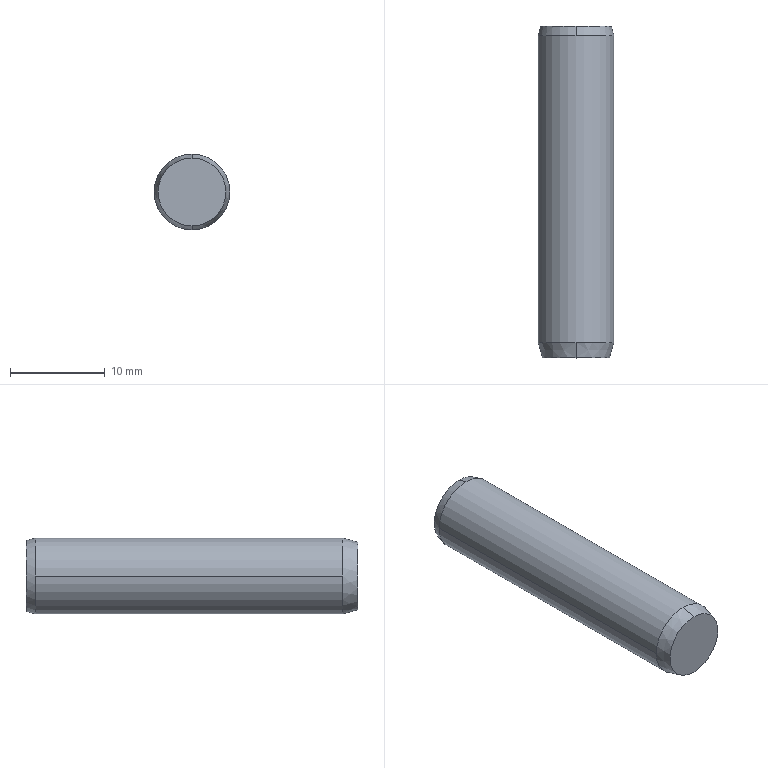Part | STEP file | 1 solid | 16 faces | box 8 x 35 x 8 mm | volume 1570 mm3 | cone 8 | cylinder 6 | plane 2 | commonest cylinder face diameters 4.134 x2 5.3 x2 8 x2
STEP:
#1=CARTESIAN_POINT('',(0.,-35.,3.571));
#2=VERTEX_POINT('',#1);
#3=CARTESIAN_POINT('',(0.,-35.,-3.571));
#4=VERTEX_POINT('',#3);
#5=CARTESIAN_POINT('',(0.,-35.,0.));
#6=DIRECTION('',(0.,1.,0.));
#7=DIRECTION('',(0.,0.,1.));
#8=AXIS2_PLACEMENT_3D('',#5,#6,#7);
#9=CIRCLE('',#8,3.571);
#10=EDGE_CURVE('',#2,#4,#9,.T.);
#11=ORIENTED_EDGE('',*,*,#10,.T.);
#12=CARTESIAN_POINT('',(0.,-33.4,-4.));
#13=VERTEX_POINT('',#12);
#14=CARTESIAN_POINT('',(0.,-35.,-3.571));
#15=DIRECTION('',(0.,0.9659,-0.2588));
#16=VECTOR('',#15,1000.);
#17=LINE('',#14,#16);
#18=EDGE_CURVE('',#4,#13,#17,.T.);
#19=ORIENTED_EDGE('',*,*,#18,.T.);
#20=CARTESIAN_POINT('',(4.,-33.4,0.));
#21=VERTEX_POINT('',#20);
#22=CARTESIAN_POINT('',(0.,-33.4,0.));
#23=DIRECTION('',(0.,1.,0.));
#24=DIRECTION('',(0.,0.,1.));
#25=AXIS2_PLACEMENT_3D('',#22,#23,#24);
#26=CIRCLE('',#25,4.);
#27=EDGE_CURVE('',#21,#13,#26,.T.);
#28=ORIENTED_EDGE('',*,*,#27,.F.);
#29=CARTESIAN_POINT('',(0.,-33.4,4.));
#30=VERTEX_POINT('',#29);
#31=CARTESIAN_POINT('',(0.,-33.4,0.));
#32=DIRECTION('',(0.,1.,0.));
#33=DIRECTION('',(0.,0.,1.));
#34=AXIS2_PLACEMENT_3D('',#31,#32,#33);
#35=CIRCLE('',#34,4.);
#36=EDGE_CURVE('',#30,#21,#35,.T.);
#37=ORIENTED_EDGE('',*,*,#36,.F.);
#38=CARTESIAN_POINT('',(0.,-35.,3.571));
#39=DIRECTION('',(0.,0.9659,0.2588));
#40=VECTOR('',#39,1000.);
#41=LINE('',#38,#40);
#42=EDGE_CURVE('',#2,#30,#41,.T.);
#43=ORIENTED_EDGE('',*,*,#42,.F.);
#44=EDGE_LOOP('',(#11,#19,#28,#37,#43));
#45=FACE_OUTER_BOUND('',#44,.T.);
#46=CARTESIAN_POINT('',(0.,-35.,0.));
#47=DIRECTION('',(0.,1.,0.));
#48=DIRECTION('',(0.,0.,1.));
#49=AXIS2_PLACEMENT_3D('',#46,#47,#48);
#50=CONICAL_SURFACE('',#49,3.571,0.2618);
#51=ADVANCED_FACE('',(#45),#50,.T.);
#52=CARTESIAN_POINT('',(-4.,-33.4,0.));
#53=VERTEX_POINT('',#52);
#54=CARTESIAN_POINT('',(0.,-33.4,0.));
#55=DIRECTION('',(0.,1.,0.));
#56=DIRECTION('',(0.,0.,1.));
#57=AXIS2_PLACEMENT_3D('',#54,#55,#56);
#58=CIRCLE('',#57,4.);
#59=EDGE_CURVE('',#53,#30,#58,.T.);
#60=ORIENTED_EDGE('',*,*,#59,.T.);
#61=ORIENTED_EDGE('',*,*,#36,.T.);
#62=CARTESIAN_POINT('',(4.,-1.,0.));
#63=VERTEX_POINT('',#62);
#64=CARTESIAN_POINT('',(4.,-13.193,0.));
#65=DIRECTION('',(0.,1.,0.));
#66=VECTOR('',#65,1000.);
#67=LINE('',#64,#66);
#68=EDGE_CURVE('',#21,#63,#67,.T.);
#69=ORIENTED_EDGE('',*,*,#68,.T.);
#70=CARTESIAN_POINT('',(0.,-1.,4.));
#71=VERTEX_POINT('',#70);
#72=CARTESIAN_POINT('',(0.,-1.,0.));
#73=DIRECTION('',(0.,1.,0.));
#74=DIRECTION('',(0.,0.,1.));
#75=AXIS2_PLACEMENT_3D('',#72,#73,#74);
#76=CIRCLE('',#75,4.);
#77=EDGE_CURVE('',#71,#63,#76,.T.);
#78=ORIENTED_EDGE('',*,*,#77,.F.);
#79=CARTESIAN_POINT('',(-4.,-1.,0.));
#80=VERTEX_POINT('',#79);
#81=CARTESIAN_POINT('',(0.,-1.,0.));
#82=DIRECTION('',(0.,1.,0.));
#83=DIRECTION('',(0.,0.,1.));
#84=AXIS2_PLACEMENT_3D('',#81,#82,#83);
#85=CIRCLE('',#84,4.);
#86=EDGE_CURVE('',#80,#71,#85,.T.);
#87=ORIENTED_EDGE('',*,*,#86,.F.);
#88=CARTESIAN_POINT('',(-4.,-13.193,0.));
#89=DIRECTION('',(0.,1.,0.));
#90=VECTOR('',#89,1000.);
#91=LINE('',#88,#90);
#92=EDGE_CURVE('',#53,#80,#91,.T.);
#93=ORIENTED_EDGE('',*,*,#92,.F.);
#94=EDGE_LOOP('',(#60,#61,#69,#78,#87,#93));
#95=FACE_OUTER_BOUND('',#94,.T.);
#96=CARTESIAN_POINT('',(0.,-13.193,0.));
#97=DIRECTION('',(0.,1.,0.));
#98=DIRECTION('',(-1.,0.,0.));
#99=AXIS2_PLACEMENT_3D('',#96,#97,#98);
#100=CYLINDRICAL_SURFACE('',#99,4.);
#101=ADVANCED_FACE('',(#95),#100,.T.);
#102=CARTESIAN_POINT('',(0.,0.,3.732));
#103=VERTEX_POINT('',#102);
#104=CARTESIAN_POINT('',(0.,0.,-3.732));
#105=VERTEX_POINT('',#104);
#106=CARTESIAN_POINT('',(0.,0.,0.));
#107=DIRECTION('',(0.,1.,0.));
#108=DIRECTION('',(0.,0.,1.));
#109=AXIS2_PLACEMENT_3D('',#106,#107,#108);
#110=CIRCLE('',#109,3.732);
#111=EDGE_CURVE('',#103,#105,#110,.T.);
#112=ORIENTED_EDGE('',*,*,#111,.F.);
#113=CARTESIAN_POINT('',(0.,-1.,4.));
#114=DIRECTION('',(0.,-0.9659,0.2588));
#115=VECTOR('',#114,1000.);
#116=LINE('',#113,#115);
#117=EDGE_CURVE('',#103,#71,#116,.T.);
#118=ORIENTED_EDGE('',*,*,#117,.T.);
#119=ORIENTED_EDGE('',*,*,#77,.T.);
#120=CARTESIAN_POINT('',(0.,-1.,-4.));
#121=VERTEX_POINT('',#120);
#122=CARTESIAN_POINT('',(0.,-1.,0.));
#123=DIRECTION('',(0.,1.,0.));
#124=DIRECTION('',(0.,0.,1.));
#125=AXIS2_PLACEMENT_3D('',#122,#123,#124);
#126=CIRCLE('',#125,4.);
#127=EDGE_CURVE('',#63,#121,#126,.T.);
#128=ORIENTED_EDGE('',*,*,#127,.T.);
#129=CARTESIAN_POINT('',(0.,-1.,-4.));
#130=DIRECTION('',(0.,-0.9659,-0.2588));
#131=VECTOR('',#130,1000.);
#132=LINE('',#129,#131);
#133=EDGE_CURVE('',#105,#121,#132,.T.);
#134=ORIENTED_EDGE('',*,*,#133,.F.);
#135=EDGE_LOOP('',(#112,#118,#119,#128,#134));
#136=FACE_OUTER_BOUND('',#135,.T.);
#137=CARTESIAN_POINT('',(0.,-1.,0.));
#138=DIRECTION('',(0.,-1.,0.));
#139=DIRECTION('',(0.,0.,-1.));
#140=AXIS2_PLACEMENT_3D('',#137,#138,#139);
#141=CONICAL_SURFACE('',#140,4.,0.2618);
#142=ADVANCED_FACE('',(#136),#141,.T.);
#143=CARTESIAN_POINT('',(0.,-13.193,0.));
#144=VERTEX_POINT('',#143);
#145=CARTESIAN_POINT('',(-2.067,-12.,0.));
#146=VERTEX_POINT('',#145);
#147=CARTESIAN_POINT('',(-2.067,-12.,0.));
#148=DIRECTION('',(-0.866,0.5,0.));
#149=VECTOR('',#148,1000.);
#150=LINE('',#147,#149);
#151=EDGE_CURVE('',#144,#146,#150,.T.);
#152=ORIENTED_EDGE('',*,*,#151,.F.);
#153=CARTESIAN_POINT('',(2.067,-12.,0.));
#154=VERTEX_POINT('',#153);
#155=CARTESIAN_POINT('',(2.067,-12.,0.));
#156=DIRECTION('',(0.866,0.5,0.));
#157=VECTOR('',#156,1000.);
#158=LINE('',#155,#157);
#159=EDGE_CURVE('',#144,#154,#158,.T.);
#160=ORIENTED_EDGE('',*,*,#159,.T.);
#161=CARTESIAN_POINT('',(0.,-12.,0.));
#162=DIRECTION('',(0.,1.,0.));
#163=DIRECTION('',(-1.,0.,0.));
#164=AXIS2_PLACEMENT_3D('',#161,#162,#163);
#165=CIRCLE('',#164,2.067);
#166=EDGE_CURVE('',#154,#146,#165,.T.);
#167=ORIENTED_EDGE('',*,*,#166,.T.);
#168=EDGE_LOOP('',(#152,#160,#167));
#169=FACE_OUTER_BOUND('',#168,.T.);
#170=CARTESIAN_POINT('',(0.,-12.,0.));
#171=DIRECTION('',(0.,1.,0.));
#172=DIRECTION('',(-1.,0.,0.));
#173=AXIS2_PLACEMENT_3D('',#170,#171,#172);
#174=CONICAL_SURFACE('',#173,2.067,1.047);
#175=ADVANCED_FACE('',(#169),#174,.F.);
#176=ORIENTED_EDGE('',*,*,#166,.F.);
#177=CARTESIAN_POINT('',(2.067,-1.537,0.));
#178=VERTEX_POINT('',#177);
#179=CARTESIAN_POINT('',(2.067,-13.193,0.));
#180=DIRECTION('',(0.,1.,0.));
#181=VECTOR('',#180,1000.);
#182=LINE('',#179,#181);
#183=EDGE_CURVE('',#154,#178,#182,.T.);
#184=ORIENTED_EDGE('',*,*,#183,.T.);
#185=CARTESIAN_POINT('',(-2.067,-1.537,0.));
#186=VERTEX_POINT('',#185);
#187=CARTESIAN_POINT('',(0.,-1.537,0.));
#188=DIRECTION('',(0.,1.,0.));
#189=DIRECTION('',(-1.,0.,0.));
#190=AXIS2_PLACEMENT_3D('',#187,#188,#189);
#191=CIRCLE('',#190,2.067);
#192=EDGE_CURVE('',#178,#186,#191,.T.);
#193=ORIENTED_EDGE('',*,*,#192,.T.);
#194=CARTESIAN_POINT('',(-2.067,-13.193,0.));
#195=DIRECTION('',(0.,1.,0.));
#196=VECTOR('',#195,1000.);
#197=LINE('',#194,#196);
#198=EDGE_CURVE('',#146,#186,#197,.T.);
#199=ORIENTED_EDGE('',*,*,#198,.F.);
#200=EDGE_LOOP('',(#176,#184,#193,#199));
#201=FACE_OUTER_BOUND('',#200,.T.);
#202=CARTESIAN_POINT('',(0.,-13.193,0.));
#203=DIRECTION('',(0.,1.,0.));
#204=DIRECTION('',(-1.,0.,0.));
#205=AXIS2_PLACEMENT_3D('',#202,#203,#204);
#206=CYLINDRICAL_SURFACE('',#205,2.067);
#207=ADVANCED_FACE('',(#201),#206,.F.);
#208=ORIENTED_EDGE('',*,*,#192,.F.);
#209=CARTESIAN_POINT('',(2.65,-1.2,0.));
#210=VERTEX_POINT('',#209);
#211=CARTESIAN_POINT('',(2.65,-1.2,0.));
#212=DIRECTION('',(0.866,0.5,0.));
#213=VECTOR('',#212,1000.);
#214=LINE('',#211,#213);
#215=EDGE_CURVE('',#178,#210,#214,.T.);
#216=ORIENTED_EDGE('',*,*,#215,.T.);
#217=CARTESIAN_POINT('',(-2.65,-1.2,0.));
#218=VERTEX_POINT('',#217);
#219=CARTESIAN_POINT('',(0.,-1.2,0.));
#220=DIRECTION('',(0.,1.,0.));
#221=DIRECTION('',(-1.,0.,0.));
#222=AXIS2_PLACEMENT_3D('',#219,#220,#221);
#223=CIRCLE('',#222,2.65);
#224=EDGE_CURVE('',#210,#218,#223,.T.);
#225=ORIENTED_EDGE('',*,*,#224,.T.);
#226=CARTESIAN_POINT('',(-2.65,-1.2,0.));
#227=DIRECTION('',(-0.866,0.5,0.));
#228=VECTOR('',#227,1000.);
#229=LINE('',#226,#228);
#230=EDGE_CURVE('',#186,#218,#229,.T.);
#231=ORIENTED_EDGE('',*,*,#230,.F.);
#232=EDGE_LOOP('',(#208,#216,#225,#231));
#233=FACE_OUTER_BOUND('',#232,.T.);
#234=CARTESIAN_POINT('',(0.,-1.2,0.));
#235=DIRECTION('',(0.,1.,0.));
#236=DIRECTION('',(-1.,0.,0.));
#237=AXIS2_PLACEMENT_3D('',#234,#235,#236);
#238=CONICAL_SURFACE('',#237,2.65,1.047);
#239=ADVANCED_FACE('',(#233),#238,.F.);
#240=ORIENTED_EDGE('',*,*,#224,.F.);
#241=CARTESIAN_POINT('',(2.65,0.,0.));
#242=VERTEX_POINT('',#241);
#243=CARTESIAN_POINT('',(2.65,-13.193,0.));
#244=DIRECTION('',(0.,1.,0.));
#245=VECTOR('',#244,1000.);
#246=LINE('',#243,#245);
#247=EDGE_CURVE('',#210,#242,#246,.T.);
#248=ORIENTED_EDGE('',*,*,#247,.T.);
#249=CARTESIAN_POINT('',(-2.65,0.,0.));
#250=VERTEX_POINT('',#249);
#251=CARTESIAN_POINT('',(0.,0.,0.));
#252=DIRECTION('',(0.,1.,0.));
#253=DIRECTION('',(-1.,0.,0.));
#254=AXIS2_PLACEMENT_3D('',#251,#252,#253);
#255=CIRCLE('',#254,2.65);
#256=EDGE_CURVE('',#242,#250,#255,.T.);
#257=ORIENTED_EDGE('',*,*,#256,.T.);
#258=CARTESIAN_POINT('',(-2.65,-13.193,0.));
#259=DIRECTION('',(0.,1.,0.));
#260=VECTOR('',#259,1000.);
#261=LINE('',#258,#260);
#262=EDGE_CURVE('',#218,#250,#261,.T.);
#263=ORIENTED_EDGE('',*,*,#262,.F.);
#264=EDGE_LOOP('',(#240,#248,#257,#263));
#265=FACE_OUTER_BOUND('',#264,.T.);
#266=CARTESIAN_POINT('',(0.,-13.193,0.));
#267=DIRECTION('',(0.,1.,0.));
#268=DIRECTION('',(-1.,0.,0.));
#269=AXIS2_PLACEMENT_3D('',#266,#267,#268);
#270=CYLINDRICAL_SURFACE('',#269,2.65);
#271=ADVANCED_FACE('',(#265),#270,.F.);
#272=CARTESIAN_POINT('',(0.,0.,0.));
#273=DIRECTION('',(0.,1.,0.));
#274=DIRECTION('',(-1.,0.,0.));
#275=AXIS2_PLACEMENT_3D('',#272,#273,#274);
#276=CIRCLE('',#275,2.65);
#277=EDGE_CURVE('',#250,#242,#276,.T.);
#278=ORIENTED_EDGE('',*,*,#277,.F.);
#279=ORIENTED_EDGE('',*,*,#256,.F.);
#280=EDGE_LOOP('',(#278,#279));
#281=FACE_BOUND('',#280,.T.);
#282=CARTESIAN_POINT('',(0.,0.,0.));
#283=DIRECTION('',(0.,1.,0.));
#284=DIRECTION('',(0.,0.,1.));
#285=AXIS2_PLACEMENT_3D('',#282,#283,#284);
#286=CIRCLE('',#285,3.732);
#287=EDGE_CURVE('',#105,#103,#286,.T.);
#288=ORIENTED_EDGE('',*,*,#287,.T.);
#289=ORIENTED_EDGE('',*,*,#111,.T.);
#290=EDGE_LOOP('',(#288,#289));
#291=FACE_OUTER_BOUND('',#290,.T.);
#292=CARTESIAN_POINT('',(4.,0.,0.));
#293=DIRECTION('',(0.,-1.,0.));
#294=DIRECTION('',(1.,0.,0.));
#295=AXIS2_PLACEMENT_3D('',#292,#293,#294);
#296=PLANE('',#295);
#297=ADVANCED_FACE('',(#281,#291),#296,.F.);
#298=ORIENTED_EDGE('',*,*,#247,.F.);
#299=CARTESIAN_POINT('',(0.,-1.2,0.));
#300=DIRECTION('',(0.,1.,0.));
#301=DIRECTION('',(-1.,0.,0.));
#302=AXIS2_PLACEMENT_3D('',#299,#300,#301);
#303=CIRCLE('',#302,2.65);
#304=EDGE_CURVE('',#218,#210,#303,.T.);
#305=ORIENTED_EDGE('',*,*,#304,.F.);
#306=ORIENTED_EDGE('',*,*,#262,.T.);
#307=ORIENTED_EDGE('',*,*,#277,.T.);
#308=EDGE_LOOP('',(#298,#305,#306,#307));
#309=FACE_OUTER_BOUND('',#308,.T.);
#310=CARTESIAN_POINT('',(0.,-13.193,0.));
#311=DIRECTION('',(0.,1.,0.));
#312=DIRECTION('',(-1.,0.,0.));
#313=AXIS2_PLACEMENT_3D('',#310,#311,#312);
#314=CYLINDRICAL_SURFACE('',#313,2.65);
#315=ADVANCED_FACE('',(#309),#314,.F.);
#316=ORIENTED_EDGE('',*,*,#215,.F.);
#317=CARTESIAN_POINT('',(0.,-1.537,0.));
#318=DIRECTION('',(0.,1.,0.));
#319=DIRECTION('',(-1.,0.,0.));
#320=AXIS2_PLACEMENT_3D('',#317,#318,#319);
#321=CIRCLE('',#320,2.067);
#322=EDGE_CURVE('',#186,#178,#321,.T.);
#323=ORIENTED_EDGE('',*,*,#322,.F.);
#324=ORIENTED_EDGE('',*,*,#230,.T.);
#325=ORIENTED_EDGE('',*,*,#304,.T.);
#326=EDGE_LOOP('',(#316,#323,#324,#325));
#327=FACE_OUTER_BOUND('',#326,.T.);
#328=CARTESIAN_POINT('',(0.,-1.2,0.));
#329=DIRECTION('',(0.,1.,0.));
#330=DIRECTION('',(-1.,0.,0.));
#331=AXIS2_PLACEMENT_3D('',#328,#329,#330);
#332=CONICAL_SURFACE('',#331,2.65,1.047);
#333=ADVANCED_FACE('',(#327),#332,.F.);
#334=ORIENTED_EDGE('',*,*,#183,.F.);
#335=CARTESIAN_POINT('',(0.,-12.,0.));
#336=DIRECTION('',(0.,1.,0.));
#337=DIRECTION('',(-1.,0.,0.));
#338=AXIS2_PLACEMENT_3D('',#335,#336,#337);
#339=CIRCLE('',#338,2.067);
#340=EDGE_CURVE('',#146,#154,#339,.T.);
#341=ORIENTED_EDGE('',*,*,#340,.F.);
#342=ORIENTED_EDGE('',*,*,#198,.T.);
#343=ORIENTED_EDGE('',*,*,#322,.T.);
#344=EDGE_LOOP('',(#334,#341,#342,#343));
#345=FACE_OUTER_BOUND('',#344,.T.);
#346=CARTESIAN_POINT('',(0.,-13.193,0.));
#347=DIRECTION('',(0.,1.,0.));
#348=DIRECTION('',(-1.,0.,0.));
#349=AXIS2_PLACEMENT_3D('',#346,#347,#348);
#350=CYLINDRICAL_SURFACE('',#349,2.067);
#351=ADVANCED_FACE('',(#345),#350,.F.);
#352=ORIENTED_EDGE('',*,*,#159,.F.);
#353=ORIENTED_EDGE('',*,*,#151,.T.);
#354=ORIENTED_EDGE('',*,*,#340,.T.);
#355=EDGE_LOOP('',(#352,#353,#354));
#356=FACE_OUTER_BOUND('',#355,.T.);
#357=CARTESIAN_POINT('',(0.,-12.,0.));
#358=DIRECTION('',(0.,1.,0.));
#359=DIRECTION('',(-1.,0.,0.));
#360=AXIS2_PLACEMENT_3D('',#357,#358,#359);
#361=CONICAL_SURFACE('',#360,2.067,1.047);
#362=ADVANCED_FACE('',(#356),#361,.F.);
#363=ORIENTED_EDGE('',*,*,#117,.F.);
#364=ORIENTED_EDGE('',*,*,#287,.F.);
#365=ORIENTED_EDGE('',*,*,#133,.T.);
#366=CARTESIAN_POINT('',(0.,-1.,0.));
#367=DIRECTION('',(0.,1.,0.));
#368=DIRECTION('',(0.,0.,1.));
#369=AXIS2_PLACEMENT_3D('',#366,#367,#368);
#370=CIRCLE('',#369,4.);
#371=EDGE_CURVE('',#121,#80,#370,.T.);
#372=ORIENTED_EDGE('',*,*,#371,.T.);
#373=ORIENTED_EDGE('',*,*,#86,.T.);
#374=EDGE_LOOP('',(#363,#364,#365,#372,#373));
#375=FACE_OUTER_BOUND('',#374,.T.);
#376=CARTESIAN_POINT('',(0.,-1.,0.));
#377=DIRECTION('',(0.,-1.,0.));
#378=DIRECTION('',(0.,0.,-1.));
#379=AXIS2_PLACEMENT_3D('',#376,#377,#378);
#380=CONICAL_SURFACE('',#379,4.,0.2618);
#381=ADVANCED_FACE('',(#375),#380,.T.);
#382=ORIENTED_EDGE('',*,*,#68,.F.);
#383=ORIENTED_EDGE('',*,*,#27,.T.);
#384=CARTESIAN_POINT('',(0.,-33.4,0.));
#385=DIRECTION('',(0.,1.,0.));
#386=DIRECTION('',(0.,0.,1.));
#387=AXIS2_PLACEMENT_3D('',#384,#385,#386);
#388=CIRCLE('',#387,4.);
#389=EDGE_CURVE('',#13,#53,#388,.T.);
#390=ORIENTED_EDGE('',*,*,#389,.T.);
#391=ORIENTED_EDGE('',*,*,#92,.T.);
#392=ORIENTED_EDGE('',*,*,#371,.F.);
#393=ORIENTED_EDGE('',*,*,#127,.F.);
#394=EDGE_LOOP('',(#382,#383,#390,#391,#392,#393));
#395=FACE_OUTER_BOUND('',#394,.T.);
#396=CARTESIAN_POINT('',(0.,-13.193,0.));
#397=DIRECTION('',(0.,1.,0.));
#398=DIRECTION('',(-1.,0.,0.));
#399=AXIS2_PLACEMENT_3D('',#396,#397,#398);
#400=CYLINDRICAL_SURFACE('',#399,4.);
#401=ADVANCED_FACE('',(#395),#400,.T.);
#402=ORIENTED_EDGE('',*,*,#18,.F.);
#403=CARTESIAN_POINT('',(0.,-35.,0.));
#404=DIRECTION('',(0.,1.,0.));
#405=DIRECTION('',(0.,0.,1.));
#406=AXIS2_PLACEMENT_3D('',#403,#404,#405);
#407=CIRCLE('',#406,3.571);
#408=EDGE_CURVE('',#4,#2,#407,.T.);
#409=ORIENTED_EDGE('',*,*,#408,.T.);
#410=ORIENTED_EDGE('',*,*,#42,.T.);
#411=ORIENTED_EDGE('',*,*,#59,.F.);
#412=ORIENTED_EDGE('',*,*,#389,.F.);
#413=EDGE_LOOP('',(#402,#409,#410,#411,#412));
#414=FACE_OUTER_BOUND('',#413,.T.);
#415=CARTESIAN_POINT('',(0.,-35.,0.));
#416=DIRECTION('',(0.,1.,0.));
#417=DIRECTION('',(0.,0.,1.));
#418=AXIS2_PLACEMENT_3D('',#415,#416,#417);
#419=CONICAL_SURFACE('',#418,3.571,0.2618);
#420=ADVANCED_FACE('',(#414),#419,.T.);
#421=ORIENTED_EDGE('',*,*,#10,.F.);
#422=ORIENTED_EDGE('',*,*,#408,.F.);
#423=EDGE_LOOP('',(#421,#422));
#424=FACE_OUTER_BOUND('',#423,.T.);
#425=CARTESIAN_POINT('',(0.,-35.,0.));
#426=DIRECTION('',(0.,1.,0.));
#427=DIRECTION('',(-1.,0.,0.));
#428=AXIS2_PLACEMENT_3D('',#425,#426,#427);
#429=PLANE('',#428);
#430=ADVANCED_FACE('',(#424),#429,.F.);
#431=CLOSED_SHELL('',(#51,#101,#142,#175,#207,#239,#271,#297,#315,#333,#351,#362,#381,#401,#420,#430));
#432=MANIFOLD_SOLID_BREP('',#431);
#433=CARTESIAN_POINT('',(0.,0.,0.));
#434=DIRECTION('',(0.,0.,1.));
#435=DIRECTION('',(1.,0.,0.));
#436=AXIS2_PLACEMENT_3D('',#433,#434,#435);
#437=(LENGTH_UNIT()NAMED_UNIT(*)SI_UNIT(.MILLI.,.METRE.));
#438=UNCERTAINTY_MEASURE_WITH_UNIT(LENGTH_MEASURE(0.00001),#437,'','');
#439=(NAMED_UNIT(*)PLANE_ANGLE_UNIT()SI_UNIT($,.RADIAN.));
#440=(NAMED_UNIT(*)SI_UNIT($,.STERADIAN.)SOLID_ANGLE_UNIT());
#441=(GEOMETRIC_REPRESENTATION_CONTEXT(3)GLOBAL_UNCERTAINTY_ASSIGNED_CONTEXT((#438))GLOBAL_UNIT_ASSIGNED_CONTEXT((#437,#439,#440))REPRESENTATION_CONTEXT('',''));
#442=ADVANCED_BREP_SHAPE_REPRESENTATION('',(#432,#436),#441);